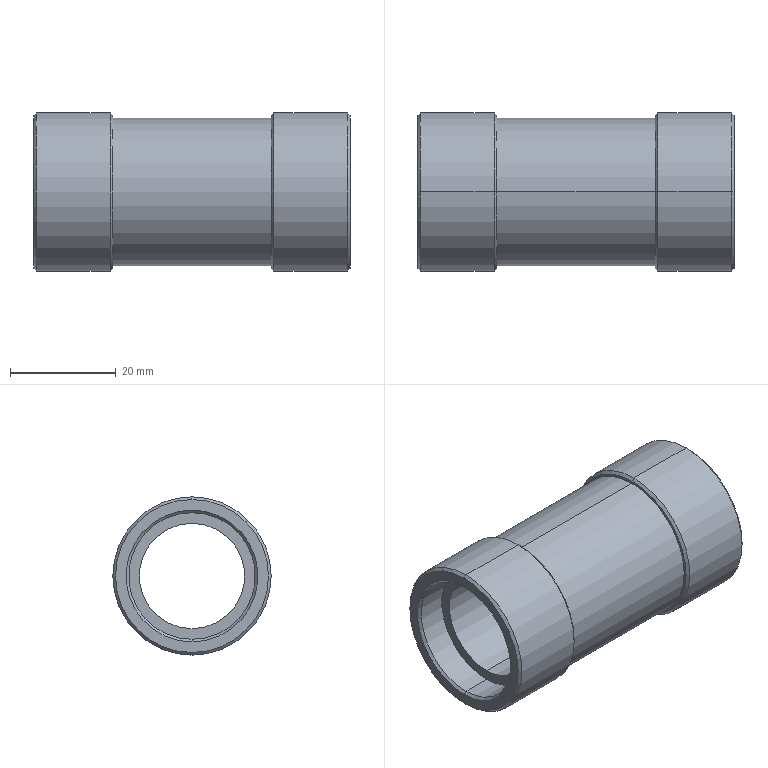Part | SolidWorks | features Chamfer 1, Revolution 1 | 1 solid | 30 faces | box 60 x 30 x 30 mm | volume 19104 mm3 | cone 12 | cylinder 12 | plane 6 | commonest cylinder face diameters 24 x4 30 x4 20 x2 28 x2
STEP:
#1=CARTESIAN_POINT('',(-15.,0.,-14.5));
#2=VERTEX_POINT('',#1);
#3=CARTESIAN_POINT('',(-15.,0.,14.5));
#4=VERTEX_POINT('',#3);
#5=CARTESIAN_POINT('',(-15.,0.,0.));
#6=DIRECTION('',(1.,0.,0.));
#7=DIRECTION('',(0.,0.,1.));
#8=AXIS2_PLACEMENT_3D('',#5,#6,#7);
#9=CIRCLE('',#8,14.5);
#10=EDGE_CURVE('',#2,#4,#9,.T.);
#11=ORIENTED_EDGE('',*,*,#10,.F.);
#12=CARTESIAN_POINT('',(-15.5,0.,-15.));
#13=VERTEX_POINT('',#12);
#14=CARTESIAN_POINT('',(-15.,0.,-14.5));
#15=DIRECTION('',(-0.7071,0.,-0.7071));
#16=VECTOR('',#15,1000.);
#17=LINE('',#14,#16);
#18=EDGE_CURVE('',#2,#13,#17,.T.);
#19=ORIENTED_EDGE('',*,*,#18,.T.);
#20=CARTESIAN_POINT('',(-15.5,0.,15.));
#21=VERTEX_POINT('',#20);
#22=CARTESIAN_POINT('',(-15.5,0.,0.));
#23=DIRECTION('',(-1.,0.,0.));
#24=DIRECTION('',(0.,0.,1.));
#25=AXIS2_PLACEMENT_3D('',#22,#23,#24);
#26=CIRCLE('',#25,15.);
#27=EDGE_CURVE('',#21,#13,#26,.T.);
#28=ORIENTED_EDGE('',*,*,#27,.F.);
#29=CARTESIAN_POINT('',(-15.,0.,14.5));
#30=DIRECTION('',(-0.7071,0.,0.7071));
#31=VECTOR('',#30,1000.);
#32=LINE('',#29,#31);
#33=EDGE_CURVE('',#4,#21,#32,.T.);
#34=ORIENTED_EDGE('',*,*,#33,.F.);
#35=EDGE_LOOP('',(#11,#19,#28,#34));
#36=FACE_OUTER_BOUND('',#35,.T.);
#37=CARTESIAN_POINT('',(-15.,0.,0.));
#38=DIRECTION('',(-1.,0.,0.));
#39=DIRECTION('',(0.,0.,1.));
#40=AXIS2_PLACEMENT_3D('',#37,#38,#39);
#41=CONICAL_SURFACE('',#40,14.5,0.7854);
#42=ADVANCED_FACE('',(#36),#41,.T.);
#43=CARTESIAN_POINT('',(15.,0.,14.5));
#44=VERTEX_POINT('',#43);
#45=CARTESIAN_POINT('',(15.,0.,-14.5));
#46=VERTEX_POINT('',#45);
#47=CARTESIAN_POINT('',(15.,0.,0.));
#48=DIRECTION('',(-1.,0.,0.));
#49=DIRECTION('',(0.,0.,1.));
#50=AXIS2_PLACEMENT_3D('',#47,#48,#49);
#51=CIRCLE('',#50,14.5);
#52=EDGE_CURVE('',#44,#46,#51,.T.);
#53=ORIENTED_EDGE('',*,*,#52,.F.);
#54=CARTESIAN_POINT('',(15.5,0.,15.));
#55=VERTEX_POINT('',#54);
#56=CARTESIAN_POINT('',(15.5,0.,15.));
#57=DIRECTION('',(0.7071,0.,0.7071));
#58=VECTOR('',#57,1000.);
#59=LINE('',#56,#58);
#60=EDGE_CURVE('',#44,#55,#59,.T.);
#61=ORIENTED_EDGE('',*,*,#60,.T.);
#62=CARTESIAN_POINT('',(15.5,0.,-15.));
#63=VERTEX_POINT('',#62);
#64=CARTESIAN_POINT('',(15.5,0.,0.));
#65=DIRECTION('',(1.,0.,0.));
#66=DIRECTION('',(0.,0.,1.));
#67=AXIS2_PLACEMENT_3D('',#64,#65,#66);
#68=CIRCLE('',#67,15.);
#69=EDGE_CURVE('',#63,#55,#68,.T.);
#70=ORIENTED_EDGE('',*,*,#69,.F.);
#71=CARTESIAN_POINT('',(15.5,0.,-15.));
#72=DIRECTION('',(0.7071,0.,-0.7071));
#73=VECTOR('',#72,1000.);
#74=LINE('',#71,#73);
#75=EDGE_CURVE('',#46,#63,#74,.T.);
#76=ORIENTED_EDGE('',*,*,#75,.F.);
#77=EDGE_LOOP('',(#53,#61,#70,#76));
#78=FACE_OUTER_BOUND('',#77,.T.);
#79=CARTESIAN_POINT('',(15.5,0.,0.));
#80=DIRECTION('',(1.,0.,0.));
#81=DIRECTION('',(0.,0.,-1.));
#82=AXIS2_PLACEMENT_3D('',#79,#80,#81);
#83=CONICAL_SURFACE('',#82,15.,0.7854);
#84=ADVANCED_FACE('',(#78),#83,.T.);
#85=CARTESIAN_POINT('',(-30.,0.,14.5));
#86=VERTEX_POINT('',#85);
#87=CARTESIAN_POINT('',(-30.,0.,-14.5));
#88=VERTEX_POINT('',#87);
#89=CARTESIAN_POINT('',(-30.,0.,0.));
#90=DIRECTION('',(-1.,0.,0.));
#91=DIRECTION('',(0.,0.,-1.));
#92=AXIS2_PLACEMENT_3D('',#89,#90,#91);
#93=CIRCLE('',#92,14.5);
#94=EDGE_CURVE('',#86,#88,#93,.T.);
#95=ORIENTED_EDGE('',*,*,#94,.F.);
#96=CARTESIAN_POINT('',(-29.5,0.,15.));
#97=VERTEX_POINT('',#96);
#98=CARTESIAN_POINT('',(-29.5,0.,15.));
#99=DIRECTION('',(0.7071,0.,0.7071));
#100=VECTOR('',#99,1000.);
#101=LINE('',#98,#100);
#102=EDGE_CURVE('',#86,#97,#101,.T.);
#103=ORIENTED_EDGE('',*,*,#102,.T.);
#104=CARTESIAN_POINT('',(-29.5,0.,-15.));
#105=VERTEX_POINT('',#104);
#106=CARTESIAN_POINT('',(-29.5,0.,0.));
#107=DIRECTION('',(1.,0.,0.));
#108=DIRECTION('',(0.,0.,-1.));
#109=AXIS2_PLACEMENT_3D('',#106,#107,#108);
#110=CIRCLE('',#109,15.);
#111=EDGE_CURVE('',#105,#97,#110,.T.);
#112=ORIENTED_EDGE('',*,*,#111,.F.);
#113=CARTESIAN_POINT('',(-29.5,0.,-15.));
#114=DIRECTION('',(0.7071,0.,-0.7071));
#115=VECTOR('',#114,1000.);
#116=LINE('',#113,#115);
#117=EDGE_CURVE('',#88,#105,#116,.T.);
#118=ORIENTED_EDGE('',*,*,#117,.F.);
#119=EDGE_LOOP('',(#95,#103,#112,#118));
#120=FACE_OUTER_BOUND('',#119,.T.);
#121=CARTESIAN_POINT('',(-29.5,0.,0.));
#122=DIRECTION('',(1.,0.,0.));
#123=DIRECTION('',(0.,0.,-1.));
#124=AXIS2_PLACEMENT_3D('',#121,#122,#123);
#125=CONICAL_SURFACE('',#124,15.,0.7854);
#126=ADVANCED_FACE('',(#120),#125,.T.);
#127=CARTESIAN_POINT('',(-29.5,0.,-12.));
#128=VERTEX_POINT('',#127);
#129=CARTESIAN_POINT('',(-29.5,0.,12.));
#130=VERTEX_POINT('',#129);
#131=CARTESIAN_POINT('',(-29.5,0.,0.));
#132=DIRECTION('',(-1.,0.,0.));
#133=DIRECTION('',(0.,0.,-1.));
#134=AXIS2_PLACEMENT_3D('',#131,#132,#133);
#135=CIRCLE('',#134,12.);
#136=EDGE_CURVE('',#128,#130,#135,.T.);
#137=ORIENTED_EDGE('',*,*,#136,.F.);
#138=CARTESIAN_POINT('',(-30.,0.,-12.5));
#139=VERTEX_POINT('',#138);
#140=CARTESIAN_POINT('',(-30.,0.,-12.5));
#141=DIRECTION('',(-0.7071,0.,-0.7071));
#142=VECTOR('',#141,1000.);
#143=LINE('',#140,#142);
#144=EDGE_CURVE('',#128,#139,#143,.T.);
#145=ORIENTED_EDGE('',*,*,#144,.T.);
#146=CARTESIAN_POINT('',(-30.,0.,12.5));
#147=VERTEX_POINT('',#146);
#148=CARTESIAN_POINT('',(-30.,0.,0.));
#149=DIRECTION('',(1.,0.,0.));
#150=DIRECTION('',(0.,0.,-1.));
#151=AXIS2_PLACEMENT_3D('',#148,#149,#150);
#152=CIRCLE('',#151,12.5);
#153=EDGE_CURVE('',#147,#139,#152,.T.);
#154=ORIENTED_EDGE('',*,*,#153,.F.);
#155=CARTESIAN_POINT('',(-30.,0.,12.5));
#156=DIRECTION('',(-0.7071,0.,0.7071));
#157=VECTOR('',#156,1000.);
#158=LINE('',#155,#157);
#159=EDGE_CURVE('',#130,#147,#158,.T.);
#160=ORIENTED_EDGE('',*,*,#159,.F.);
#161=EDGE_LOOP('',(#137,#145,#154,#160));
#162=FACE_OUTER_BOUND('',#161,.T.);
#163=CARTESIAN_POINT('',(-30.,0.,0.));
#164=DIRECTION('',(-1.,0.,0.));
#165=DIRECTION('',(0.,0.,1.));
#166=AXIS2_PLACEMENT_3D('',#163,#164,#165);
#167=CONICAL_SURFACE('',#166,12.5,0.7854);
#168=ADVANCED_FACE('',(#162),#167,.F.);
#169=CARTESIAN_POINT('',(30.,0.,-14.5));
#170=VERTEX_POINT('',#169);
#171=CARTESIAN_POINT('',(30.,0.,14.5));
#172=VERTEX_POINT('',#171);
#173=CARTESIAN_POINT('',(30.,0.,0.));
#174=DIRECTION('',(1.,0.,0.));
#175=DIRECTION('',(0.,0.,-1.));
#176=AXIS2_PLACEMENT_3D('',#173,#174,#175);
#177=CIRCLE('',#176,14.5);
#178=EDGE_CURVE('',#170,#172,#177,.T.);
#179=ORIENTED_EDGE('',*,*,#178,.F.);
#180=CARTESIAN_POINT('',(29.5,0.,-15.));
#181=VERTEX_POINT('',#180);
#182=CARTESIAN_POINT('',(30.,0.,-14.5));
#183=DIRECTION('',(-0.7071,0.,-0.7071));
#184=VECTOR('',#183,1000.);
#185=LINE('',#182,#184);
#186=EDGE_CURVE('',#170,#181,#185,.T.);
#187=ORIENTED_EDGE('',*,*,#186,.T.);
#188=CARTESIAN_POINT('',(29.5,0.,15.));
#189=VERTEX_POINT('',#188);
#190=CARTESIAN_POINT('',(29.5,0.,0.));
#191=DIRECTION('',(-1.,0.,0.));
#192=DIRECTION('',(0.,0.,-1.));
#193=AXIS2_PLACEMENT_3D('',#190,#191,#192);
#194=CIRCLE('',#193,15.);
#195=EDGE_CURVE('',#189,#181,#194,.T.);
#196=ORIENTED_EDGE('',*,*,#195,.F.);
#197=CARTESIAN_POINT('',(30.,0.,14.5));
#198=DIRECTION('',(-0.7071,0.,0.7071));
#199=VECTOR('',#198,1000.);
#200=LINE('',#197,#199);
#201=EDGE_CURVE('',#172,#189,#200,.T.);
#202=ORIENTED_EDGE('',*,*,#201,.F.);
#203=EDGE_LOOP('',(#179,#187,#196,#202));
#204=FACE_OUTER_BOUND('',#203,.T.);
#205=CARTESIAN_POINT('',(30.,0.,0.));
#206=DIRECTION('',(-1.,0.,0.));
#207=DIRECTION('',(0.,0.,1.));
#208=AXIS2_PLACEMENT_3D('',#205,#206,#207);
#209=CONICAL_SURFACE('',#208,14.5,0.7854);
#210=ADVANCED_FACE('',(#204),#209,.T.);
#211=CARTESIAN_POINT('',(29.5,0.,12.));
#212=VERTEX_POINT('',#211);
#213=CARTESIAN_POINT('',(29.5,0.,-12.));
#214=VERTEX_POINT('',#213);
#215=CARTESIAN_POINT('',(29.5,0.,0.));
#216=DIRECTION('',(1.,0.,0.));
#217=DIRECTION('',(0.,0.,-1.));
#218=AXIS2_PLACEMENT_3D('',#215,#216,#217);
#219=CIRCLE('',#218,12.);
#220=EDGE_CURVE('',#212,#214,#219,.T.);
#221=ORIENTED_EDGE('',*,*,#220,.F.);
#222=CARTESIAN_POINT('',(30.,0.,12.5));
#223=VERTEX_POINT('',#222);
#224=CARTESIAN_POINT('',(29.5,0.,12.));
#225=DIRECTION('',(0.7071,0.,0.7071));
#226=VECTOR('',#225,1000.);
#227=LINE('',#224,#226);
#228=EDGE_CURVE('',#212,#223,#227,.T.);
#229=ORIENTED_EDGE('',*,*,#228,.T.);
#230=CARTESIAN_POINT('',(30.,0.,-12.5));
#231=VERTEX_POINT('',#230);
#232=CARTESIAN_POINT('',(30.,0.,0.));
#233=DIRECTION('',(-1.,0.,0.));
#234=DIRECTION('',(0.,0.,-1.));
#235=AXIS2_PLACEMENT_3D('',#232,#233,#234);
#236=CIRCLE('',#235,12.5);
#237=EDGE_CURVE('',#231,#223,#236,.T.);
#238=ORIENTED_EDGE('',*,*,#237,.F.);
#239=CARTESIAN_POINT('',(29.5,0.,-12.));
#240=DIRECTION('',(0.7071,0.,-0.7071));
#241=VECTOR('',#240,1000.);
#242=LINE('',#239,#241);
#243=EDGE_CURVE('',#214,#231,#242,.T.);
#244=ORIENTED_EDGE('',*,*,#243,.F.);
#245=EDGE_LOOP('',(#221,#229,#238,#244));
#246=FACE_OUTER_BOUND('',#245,.T.);
#247=CARTESIAN_POINT('',(29.5,0.,0.));
#248=DIRECTION('',(1.,0.,0.));
#249=DIRECTION('',(0.,0.,-1.));
#250=AXIS2_PLACEMENT_3D('',#247,#248,#249);
#251=CONICAL_SURFACE('',#250,12.,0.7854);
#252=ADVANCED_FACE('',(#246),#251,.F.);
#253=CARTESIAN_POINT('',(24.,0.,12.));
#254=VERTEX_POINT('',#253);
#255=CARTESIAN_POINT('',(24.,0.,-12.));
#256=VERTEX_POINT('',#255);
#257=CARTESIAN_POINT('',(24.,0.,0.));
#258=DIRECTION('',(1.,0.,0.));
#259=DIRECTION('',(0.,0.,-1.));
#260=AXIS2_PLACEMENT_3D('',#257,#258,#259);
#261=CIRCLE('',#260,12.);
#262=EDGE_CURVE('',#254,#256,#261,.T.);
#263=ORIENTED_EDGE('',*,*,#262,.F.);
#264=CARTESIAN_POINT('',(48.534,0.,12.));
#265=DIRECTION('',(1.,0.,0.));
#266=VECTOR('',#265,1000.);
#267=LINE('',#264,#266);
#268=EDGE_CURVE('',#254,#212,#267,.T.);
#269=ORIENTED_EDGE('',*,*,#268,.T.);
#270=ORIENTED_EDGE('',*,*,#220,.T.);
#271=CARTESIAN_POINT('',(48.534,0.,-12.));
#272=DIRECTION('',(1.,0.,0.));
#273=VECTOR('',#272,1000.);
#274=LINE('',#271,#273);
#275=EDGE_CURVE('',#256,#214,#274,.T.);
#276=ORIENTED_EDGE('',*,*,#275,.F.);
#277=EDGE_LOOP('',(#263,#269,#270,#276));
#278=FACE_OUTER_BOUND('',#277,.T.);
#279=CARTESIAN_POINT('',(48.534,0.,0.));
#280=DIRECTION('',(1.,0.,0.));
#281=DIRECTION('',(0.,0.,-1.));
#282=AXIS2_PLACEMENT_3D('',#279,#280,#281);
#283=CYLINDRICAL_SURFACE('',#282,12.);
#284=ADVANCED_FACE('',(#278),#283,.F.);
#285=CARTESIAN_POINT('',(-24.,0.,10.));
#286=VERTEX_POINT('',#285);
#287=CARTESIAN_POINT('',(-24.,0.,-10.));
#288=VERTEX_POINT('',#287);
#289=CARTESIAN_POINT('',(-24.,0.,0.));
#290=DIRECTION('',(1.,0.,0.));
#291=DIRECTION('',(0.,0.,-1.));
#292=AXIS2_PLACEMENT_3D('',#289,#290,#291);
#293=CIRCLE('',#292,10.);
#294=EDGE_CURVE('',#286,#288,#293,.T.);
#295=ORIENTED_EDGE('',*,*,#294,.F.);
#296=CARTESIAN_POINT('',(24.,0.,10.));
#297=VERTEX_POINT('',#296);
#298=CARTESIAN_POINT('',(48.534,0.,10.));
#299=DIRECTION('',(1.,0.,0.));
#300=VECTOR('',#299,1000.);
#301=LINE('',#298,#300);
#302=EDGE_CURVE('',#286,#297,#301,.T.);
#303=ORIENTED_EDGE('',*,*,#302,.T.);
#304=CARTESIAN_POINT('',(24.,0.,-10.));
#305=VERTEX_POINT('',#304);
#306=CARTESIAN_POINT('',(24.,0.,0.));
#307=DIRECTION('',(1.,0.,0.));
#308=DIRECTION('',(0.,0.,-1.));
#309=AXIS2_PLACEMENT_3D('',#306,#307,#308);
#310=CIRCLE('',#309,10.);
#311=EDGE_CURVE('',#297,#305,#310,.T.);
#312=ORIENTED_EDGE('',*,*,#311,.T.);
#313=CARTESIAN_POINT('',(48.534,0.,-10.));
#314=DIRECTION('',(1.,0.,0.));
#315=VECTOR('',#314,1000.);
#316=LINE('',#313,#315);
#317=EDGE_CURVE('',#288,#305,#316,.T.);
#318=ORIENTED_EDGE('',*,*,#317,.F.);
#319=EDGE_LOOP('',(#295,#303,#312,#318));
#320=FACE_OUTER_BOUND('',#319,.T.);
#321=CARTESIAN_POINT('',(48.534,0.,0.));
#322=DIRECTION('',(1.,0.,0.));
#323=DIRECTION('',(0.,0.,-1.));
#324=AXIS2_PLACEMENT_3D('',#321,#322,#323);
#325=CYLINDRICAL_SURFACE('',#324,10.);
#326=ADVANCED_FACE('',(#320),#325,.F.);
#327=ORIENTED_EDGE('',*,*,#136,.T.);
#328=CARTESIAN_POINT('',(-24.,0.,12.));
#329=VERTEX_POINT('',#328);
#330=CARTESIAN_POINT('',(48.534,0.,12.));
#331=DIRECTION('',(1.,0.,0.));
#332=VECTOR('',#331,1000.);
#333=LINE('',#330,#332);
#334=EDGE_CURVE('',#130,#329,#333,.T.);
#335=ORIENTED_EDGE('',*,*,#334,.T.);
#336=CARTESIAN_POINT('',(-24.,0.,-12.));
#337=VERTEX_POINT('',#336);
#338=CARTESIAN_POINT('',(-24.,0.,0.));
#339=DIRECTION('',(1.,0.,0.));
#340=DIRECTION('',(0.,0.,-1.));
#341=AXIS2_PLACEMENT_3D('',#338,#339,#340);
#342=CIRCLE('',#341,12.);
#343=EDGE_CURVE('',#329,#337,#342,.T.);
#344=ORIENTED_EDGE('',*,*,#343,.T.);
#345=CARTESIAN_POINT('',(48.534,0.,-12.));
#346=DIRECTION('',(1.,0.,0.));
#347=VECTOR('',#346,1000.);
#348=LINE('',#345,#347);
#349=EDGE_CURVE('',#128,#337,#348,.T.);
#350=ORIENTED_EDGE('',*,*,#349,.F.);
#351=EDGE_LOOP('',(#327,#335,#344,#350));
#352=FACE_OUTER_BOUND('',#351,.T.);
#353=CARTESIAN_POINT('',(48.534,0.,0.));
#354=DIRECTION('',(1.,0.,0.));
#355=DIRECTION('',(0.,0.,-1.));
#356=AXIS2_PLACEMENT_3D('',#353,#354,#355);
#357=CYLINDRICAL_SURFACE('',#356,12.);
#358=ADVANCED_FACE('',(#352),#357,.F.);
#359=ORIENTED_EDGE('',*,*,#111,.T.);
#360=CARTESIAN_POINT('',(48.534,0.,15.));
#361=DIRECTION('',(1.,0.,0.));
#362=VECTOR('',#361,1000.);
#363=LINE('',#360,#362);
#364=EDGE_CURVE('',#97,#21,#363,.T.);
#365=ORIENTED_EDGE('',*,*,#364,.T.);
#366=ORIENTED_EDGE('',*,*,#27,.T.);
#367=CARTESIAN_POINT('',(48.534,0.,-15.));
#368=DIRECTION('',(1.,0.,0.));
#369=VECTOR('',#368,1000.);
#370=LINE('',#367,#369);
#371=EDGE_CURVE('',#105,#13,#370,.T.);
#372=ORIENTED_EDGE('',*,*,#371,.F.);
#373=EDGE_LOOP('',(#359,#365,#366,#372));
#374=FACE_OUTER_BOUND('',#373,.T.);
#375=CARTESIAN_POINT('',(48.534,0.,0.));
#376=DIRECTION('',(1.,0.,0.));
#377=DIRECTION('',(0.,0.,-1.));
#378=AXIS2_PLACEMENT_3D('',#375,#376,#377);
#379=CYLINDRICAL_SURFACE('',#378,15.);
#380=ADVANCED_FACE('',(#374),#379,.T.);
#381=CARTESIAN_POINT('',(-15.,0.,-14.));
#382=VERTEX_POINT('',#381);
#383=CARTESIAN_POINT('',(-15.,0.,14.));
#384=VERTEX_POINT('',#383);
#385=CARTESIAN_POINT('',(-15.,0.,0.));
#386=DIRECTION('',(1.,0.,0.));
#387=DIRECTION('',(0.,0.,-1.));
#388=AXIS2_PLACEMENT_3D('',#385,#386,#387);
#389=CIRCLE('',#388,14.);
#390=EDGE_CURVE('',#382,#384,#389,.T.);
#391=ORIENTED_EDGE('',*,*,#390,.T.);
#392=CARTESIAN_POINT('',(15.,0.,14.));
#393=VERTEX_POINT('',#392);
#394=CARTESIAN_POINT('',(48.534,0.,14.));
#395=DIRECTION('',(1.,0.,0.));
#396=VECTOR('',#395,1000.);
#397=LINE('',#394,#396);
#398=EDGE_CURVE('',#384,#393,#397,.T.);
#399=ORIENTED_EDGE('',*,*,#398,.T.);
#400=CARTESIAN_POINT('',(15.,0.,-14.));
#401=VERTEX_POINT('',#400);
#402=CARTESIAN_POINT('',(15.,0.,0.));
#403=DIRECTION('',(1.,0.,0.));
#404=DIRECTION('',(0.,0.,-1.));
#405=AXIS2_PLACEMENT_3D('',#402,#403,#404);
#406=CIRCLE('',#405,14.);
#407=EDGE_CURVE('',#401,#393,#406,.T.);
#408=ORIENTED_EDGE('',*,*,#407,.F.);
#409=CARTESIAN_POINT('',(48.534,0.,-14.));
#410=DIRECTION('',(1.,0.,0.));
#411=VECTOR('',#410,1000.);
#412=LINE('',#409,#411);
#413=EDGE_CURVE('',#382,#401,#412,.T.);
#414=ORIENTED_EDGE('',*,*,#413,.F.);
#415=EDGE_LOOP('',(#391,#399,#408,#414));
#416=FACE_OUTER_BOUND('',#415,.T.);
#417=CARTESIAN_POINT('',(48.534,0.,0.));
#418=DIRECTION('',(1.,0.,0.));
#419=DIRECTION('',(0.,0.,-1.));
#420=AXIS2_PLACEMENT_3D('',#417,#418,#419);
#421=CYLINDRICAL_SURFACE('',#420,14.);
#422=ADVANCED_FACE('',(#416),#421,.T.);
#423=ORIENTED_EDGE('',*,*,#69,.T.);
#424=CARTESIAN_POINT('',(48.534,0.,15.));
#425=DIRECTION('',(1.,0.,0.));
#426=VECTOR('',#425,1000.);
#427=LINE('',#424,#426);
#428=EDGE_CURVE('',#55,#189,#427,.T.);
#429=ORIENTED_EDGE('',*,*,#428,.T.);
#430=ORIENTED_EDGE('',*,*,#195,.T.);
#431=CARTESIAN_POINT('',(48.534,0.,-15.));
#432=DIRECTION('',(1.,0.,0.));
#433=VECTOR('',#432,1000.);
#434=LINE('',#431,#433);
#435=EDGE_CURVE('',#63,#181,#434,.T.);
#436=ORIENTED_EDGE('',*,*,#435,.F.);
#437=EDGE_LOOP('',(#423,#429,#430,#436));
#438=FACE_OUTER_BOUND('',#437,.T.);
#439=CARTESIAN_POINT('',(48.534,0.,0.));
#440=DIRECTION('',(1.,0.,0.));
#441=DIRECTION('',(0.,0.,-1.));
#442=AXIS2_PLACEMENT_3D('',#439,#440,#441);
#443=CYLINDRICAL_SURFACE('',#442,15.);
#444=ADVANCED_FACE('',(#438),#443,.T.);
#445=ORIENTED_EDGE('',*,*,#428,.F.);
#446=CARTESIAN_POINT('',(15.5,0.,0.));
#447=DIRECTION('',(1.,0.,0.));
#448=DIRECTION('',(0.,0.,1.));
#449=AXIS2_PLACEMENT_3D('',#446,#447,#448);
#450=CIRCLE('',#449,15.);
#451=EDGE_CURVE('',#55,#63,#450,.T.);
#452=ORIENTED_EDGE('',*,*,#451,.T.);
#453=ORIENTED_EDGE('',*,*,#435,.T.);
#454=CARTESIAN_POINT('',(29.5,0.,0.));
#455=DIRECTION('',(-1.,0.,0.));
#456=DIRECTION('',(0.,0.,-1.));
#457=AXIS2_PLACEMENT_3D('',#454,#455,#456);
#458=CIRCLE('',#457,15.);
#459=EDGE_CURVE('',#181,#189,#458,.T.);
#460=ORIENTED_EDGE('',*,*,#459,.T.);
#461=EDGE_LOOP('',(#445,#452,#453,#460));
#462=FACE_OUTER_BOUND('',#461,.T.);
#463=CARTESIAN_POINT('',(48.534,0.,0.));
#464=DIRECTION('',(1.,0.,0.));
#465=DIRECTION('',(0.,0.,-1.));
#466=AXIS2_PLACEMENT_3D('',#463,#464,#465);
#467=CYLINDRICAL_SURFACE('',#466,15.);
#468=ADVANCED_FACE('',(#462),#467,.T.);
#469=CARTESIAN_POINT('',(15.,0.,0.));
#470=DIRECTION('',(-1.,0.,0.));
#471=DIRECTION('',(0.,0.,1.));
#472=AXIS2_PLACEMENT_3D('',#469,#470,#471);
#473=CIRCLE('',#472,14.5);
#474=EDGE_CURVE('',#46,#44,#473,.T.);
#475=ORIENTED_EDGE('',*,*,#474,.T.);
#476=ORIENTED_EDGE('',*,*,#52,.T.);
#477=EDGE_LOOP('',(#475,#476));
#478=FACE_OUTER_BOUND('',#477,.T.);
#479=ORIENTED_EDGE('',*,*,#407,.T.);
#480=CARTESIAN_POINT('',(15.,0.,0.));
#481=DIRECTION('',(1.,0.,0.));
#482=DIRECTION('',(0.,0.,-1.));
#483=AXIS2_PLACEMENT_3D('',#480,#481,#482);
#484=CIRCLE('',#483,14.);
#485=EDGE_CURVE('',#393,#401,#484,.T.);
#486=ORIENTED_EDGE('',*,*,#485,.T.);
#487=EDGE_LOOP('',(#479,#486));
#488=FACE_BOUND('',#487,.T.);
#489=CARTESIAN_POINT('',(15.,0.,0.));
#490=DIRECTION('',(-1.,0.,0.));
#491=DIRECTION('',(0.,0.,1.));
#492=AXIS2_PLACEMENT_3D('',#489,#490,#491);
#493=PLANE('',#492);
#494=ADVANCED_FACE('',(#478,#488),#493,.T.);
#495=ORIENTED_EDGE('',*,*,#398,.F.);
#496=CARTESIAN_POINT('',(-15.,0.,0.));
#497=DIRECTION('',(1.,0.,0.));
#498=DIRECTION('',(0.,0.,-1.));
#499=AXIS2_PLACEMENT_3D('',#496,#497,#498);
#500=CIRCLE('',#499,14.);
#501=EDGE_CURVE('',#384,#382,#500,.T.);
#502=ORIENTED_EDGE('',*,*,#501,.T.);
#503=ORIENTED_EDGE('',*,*,#413,.T.);
#504=ORIENTED_EDGE('',*,*,#485,.F.);
#505=EDGE_LOOP('',(#495,#502,#503,#504));
#506=FACE_OUTER_BOUND('',#505,.T.);
#507=CARTESIAN_POINT('',(48.534,0.,0.));
#508=DIRECTION('',(1.,0.,0.));
#509=DIRECTION('',(0.,0.,-1.));
#510=AXIS2_PLACEMENT_3D('',#507,#508,#509);
#511=CYLINDRICAL_SURFACE('',#510,14.);
#512=ADVANCED_FACE('',(#506),#511,.T.);
#513=CARTESIAN_POINT('',(-15.,0.,0.));
#514=DIRECTION('',(1.,0.,0.));
#515=DIRECTION('',(0.,0.,1.));
#516=AXIS2_PLACEMENT_3D('',#513,#514,#515);
#517=CIRCLE('',#516,14.5);
#518=EDGE_CURVE('',#4,#2,#517,.T.);
#519=ORIENTED_EDGE('',*,*,#518,.T.);
#520=ORIENTED_EDGE('',*,*,#10,.T.);
#521=EDGE_LOOP('',(#519,#520));
#522=FACE_OUTER_BOUND('',#521,.T.);
#523=ORIENTED_EDGE('',*,*,#390,.F.);
#524=ORIENTED_EDGE('',*,*,#501,.F.);
#525=EDGE_LOOP('',(#523,#524));
#526=FACE_BOUND('',#525,.T.);
#527=CARTESIAN_POINT('',(-15.,0.,0.));
#528=DIRECTION('',(-1.,0.,0.));
#529=DIRECTION('',(0.,0.,1.));
#530=AXIS2_PLACEMENT_3D('',#527,#528,#529);
#531=PLANE('',#530);
#532=ADVANCED_FACE('',(#522,#526),#531,.F.);
#533=ORIENTED_EDGE('',*,*,#364,.F.);
#534=CARTESIAN_POINT('',(-29.5,0.,0.));
#535=DIRECTION('',(1.,0.,0.));
#536=DIRECTION('',(0.,0.,-1.));
#537=AXIS2_PLACEMENT_3D('',#534,#535,#536);
#538=CIRCLE('',#537,15.);
#539=EDGE_CURVE('',#97,#105,#538,.T.);
#540=ORIENTED_EDGE('',*,*,#539,.T.);
#541=ORIENTED_EDGE('',*,*,#371,.T.);
#542=CARTESIAN_POINT('',(-15.5,0.,0.));
#543=DIRECTION('',(-1.,0.,0.));
#544=DIRECTION('',(0.,0.,1.));
#545=AXIS2_PLACEMENT_3D('',#542,#543,#544);
#546=CIRCLE('',#545,15.);
#547=EDGE_CURVE('',#13,#21,#546,.T.);
#548=ORIENTED_EDGE('',*,*,#547,.T.);
#549=EDGE_LOOP('',(#533,#540,#541,#548));
#550=FACE_OUTER_BOUND('',#549,.T.);
#551=CARTESIAN_POINT('',(48.534,0.,0.));
#552=DIRECTION('',(1.,0.,0.));
#553=DIRECTION('',(0.,0.,-1.));
#554=AXIS2_PLACEMENT_3D('',#551,#552,#553);
#555=CYLINDRICAL_SURFACE('',#554,15.);
#556=ADVANCED_FACE('',(#550),#555,.T.);
#557=ORIENTED_EDGE('',*,*,#153,.T.);
#558=CARTESIAN_POINT('',(-30.,0.,0.));
#559=DIRECTION('',(1.,0.,0.));
#560=DIRECTION('',(0.,0.,-1.));
#561=AXIS2_PLACEMENT_3D('',#558,#559,#560);
#562=CIRCLE('',#561,12.5);
#563=EDGE_CURVE('',#139,#147,#562,.T.);
#564=ORIENTED_EDGE('',*,*,#563,.T.);
#565=EDGE_LOOP('',(#557,#564));
#566=FACE_BOUND('',#565,.T.);
#567=CARTESIAN_POINT('',(-30.,0.,0.));
#568=DIRECTION('',(-1.,0.,0.));
#569=DIRECTION('',(0.,0.,-1.));
#570=AXIS2_PLACEMENT_3D('',#567,#568,#569);
#571=CIRCLE('',#570,14.5);
#572=EDGE_CURVE('',#88,#86,#571,.T.);
#573=ORIENTED_EDGE('',*,*,#572,.T.);
#574=ORIENTED_EDGE('',*,*,#94,.T.);
#575=EDGE_LOOP('',(#573,#574));
#576=FACE_OUTER_BOUND('',#575,.T.);
#577=CARTESIAN_POINT('',(-30.,0.,0.));
#578=DIRECTION('',(1.,0.,0.));
#579=DIRECTION('',(0.,0.,-1.));
#580=AXIS2_PLACEMENT_3D('',#577,#578,#579);
#581=PLANE('',#580);
#582=ADVANCED_FACE('',(#566,#576),#581,.F.);
#583=ORIENTED_EDGE('',*,*,#334,.F.);
#584=CARTESIAN_POINT('',(-29.5,0.,0.));
#585=DIRECTION('',(-1.,0.,0.));
#586=DIRECTION('',(0.,0.,-1.));
#587=AXIS2_PLACEMENT_3D('',#584,#585,#586);
#588=CIRCLE('',#587,12.);
#589=EDGE_CURVE('',#130,#128,#588,.T.);
#590=ORIENTED_EDGE('',*,*,#589,.T.);
#591=ORIENTED_EDGE('',*,*,#349,.T.);
#592=CARTESIAN_POINT('',(-24.,0.,0.));
#593=DIRECTION('',(1.,0.,0.));
#594=DIRECTION('',(0.,0.,-1.));
#595=AXIS2_PLACEMENT_3D('',#592,#593,#594);
#596=CIRCLE('',#595,12.);
#597=EDGE_CURVE('',#337,#329,#596,.T.);
#598=ORIENTED_EDGE('',*,*,#597,.T.);
#599=EDGE_LOOP('',(#583,#590,#591,#598));
#600=FACE_OUTER_BOUND('',#599,.T.);
#601=CARTESIAN_POINT('',(48.534,0.,0.));
#602=DIRECTION('',(1.,0.,0.));
#603=DIRECTION('',(0.,0.,-1.));
#604=AXIS2_PLACEMENT_3D('',#601,#602,#603);
#605=CYLINDRICAL_SURFACE('',#604,12.);
#606=ADVANCED_FACE('',(#600),#605,.F.);
#607=ORIENTED_EDGE('',*,*,#597,.F.);
#608=ORIENTED_EDGE('',*,*,#343,.F.);
#609=EDGE_LOOP('',(#607,#608));
#610=FACE_OUTER_BOUND('',#609,.T.);
#611=CARTESIAN_POINT('',(-24.,0.,0.));
#612=DIRECTION('',(1.,0.,0.));
#613=DIRECTION('',(0.,0.,-1.));
#614=AXIS2_PLACEMENT_3D('',#611,#612,#613);
#615=CIRCLE('',#614,10.);
#616=EDGE_CURVE('',#288,#286,#615,.T.);
#617=ORIENTED_EDGE('',*,*,#616,.T.);
#618=ORIENTED_EDGE('',*,*,#294,.T.);
#619=EDGE_LOOP('',(#617,#618));
#620=FACE_BOUND('',#619,.T.);
#621=CARTESIAN_POINT('',(-24.,0.,0.));
#622=DIRECTION('',(1.,0.,0.));
#623=DIRECTION('',(0.,0.,-1.));
#624=AXIS2_PLACEMENT_3D('',#621,#622,#623);
#625=PLANE('',#624);
#626=ADVANCED_FACE('',(#610,#620),#625,.F.);
#627=ORIENTED_EDGE('',*,*,#302,.F.);
#628=ORIENTED_EDGE('',*,*,#616,.F.);
#629=ORIENTED_EDGE('',*,*,#317,.T.);
#630=CARTESIAN_POINT('',(24.,0.,0.));
#631=DIRECTION('',(1.,0.,0.));
#632=DIRECTION('',(0.,0.,-1.));
#633=AXIS2_PLACEMENT_3D('',#630,#631,#632);
#634=CIRCLE('',#633,10.);
#635=EDGE_CURVE('',#305,#297,#634,.T.);
#636=ORIENTED_EDGE('',*,*,#635,.T.);
#637=EDGE_LOOP('',(#627,#628,#629,#636));
#638=FACE_OUTER_BOUND('',#637,.T.);
#639=CARTESIAN_POINT('',(48.534,0.,0.));
#640=DIRECTION('',(1.,0.,0.));
#641=DIRECTION('',(0.,0.,-1.));
#642=AXIS2_PLACEMENT_3D('',#639,#640,#641);
#643=CYLINDRICAL_SURFACE('',#642,10.);
#644=ADVANCED_FACE('',(#638),#643,.F.);
#645=CARTESIAN_POINT('',(24.,0.,0.));
#646=DIRECTION('',(1.,0.,0.));
#647=DIRECTION('',(0.,0.,-1.));
#648=AXIS2_PLACEMENT_3D('',#645,#646,#647);
#649=CIRCLE('',#648,12.);
#650=EDGE_CURVE('',#256,#254,#649,.T.);
#651=ORIENTED_EDGE('',*,*,#650,.T.);
#652=ORIENTED_EDGE('',*,*,#262,.T.);
#653=EDGE_LOOP('',(#651,#652));
#654=FACE_OUTER_BOUND('',#653,.T.);
#655=ORIENTED_EDGE('',*,*,#635,.F.);
#656=ORIENTED_EDGE('',*,*,#311,.F.);
#657=EDGE_LOOP('',(#655,#656));
#658=FACE_BOUND('',#657,.T.);
#659=CARTESIAN_POINT('',(24.,0.,0.));
#660=DIRECTION('',(1.,0.,0.));
#661=DIRECTION('',(0.,0.,-1.));
#662=AXIS2_PLACEMENT_3D('',#659,#660,#661);
#663=PLANE('',#662);
#664=ADVANCED_FACE('',(#654,#658),#663,.T.);
#665=ORIENTED_EDGE('',*,*,#268,.F.);
#666=ORIENTED_EDGE('',*,*,#650,.F.);
#667=ORIENTED_EDGE('',*,*,#275,.T.);
#668=CARTESIAN_POINT('',(29.5,0.,0.));
#669=DIRECTION('',(1.,0.,0.));
#670=DIRECTION('',(0.,0.,-1.));
#671=AXIS2_PLACEMENT_3D('',#668,#669,#670);
#672=CIRCLE('',#671,12.);
#673=EDGE_CURVE('',#214,#212,#672,.T.);
#674=ORIENTED_EDGE('',*,*,#673,.T.);
#675=EDGE_LOOP('',(#665,#666,#667,#674));
#676=FACE_OUTER_BOUND('',#675,.T.);
#677=CARTESIAN_POINT('',(48.534,0.,0.));
#678=DIRECTION('',(1.,0.,0.));
#679=DIRECTION('',(0.,0.,-1.));
#680=AXIS2_PLACEMENT_3D('',#677,#678,#679);
#681=CYLINDRICAL_SURFACE('',#680,12.);
#682=ADVANCED_FACE('',(#676),#681,.F.);
#683=ORIENTED_EDGE('',*,*,#237,.T.);
#684=CARTESIAN_POINT('',(30.,0.,0.));
#685=DIRECTION('',(-1.,0.,0.));
#686=DIRECTION('',(0.,0.,-1.));
#687=AXIS2_PLACEMENT_3D('',#684,#685,#686);
#688=CIRCLE('',#687,12.5);
#689=EDGE_CURVE('',#223,#231,#688,.T.);
#690=ORIENTED_EDGE('',*,*,#689,.T.);
#691=EDGE_LOOP('',(#683,#690));
#692=FACE_BOUND('',#691,.T.);
#693=CARTESIAN_POINT('',(30.,0.,0.));
#694=DIRECTION('',(1.,0.,0.));
#695=DIRECTION('',(0.,0.,-1.));
#696=AXIS2_PLACEMENT_3D('',#693,#694,#695);
#697=CIRCLE('',#696,14.5);
#698=EDGE_CURVE('',#172,#170,#697,.T.);
#699=ORIENTED_EDGE('',*,*,#698,.T.);
#700=ORIENTED_EDGE('',*,*,#178,.T.);
#701=EDGE_LOOP('',(#699,#700));
#702=FACE_OUTER_BOUND('',#701,.T.);
#703=CARTESIAN_POINT('',(30.,0.,0.));
#704=DIRECTION('',(1.,0.,0.));
#705=DIRECTION('',(0.,0.,-1.));
#706=AXIS2_PLACEMENT_3D('',#703,#704,#705);
#707=PLANE('',#706);
#708=ADVANCED_FACE('',(#692,#702),#707,.T.);
#709=ORIENTED_EDGE('',*,*,#228,.F.);
#710=ORIENTED_EDGE('',*,*,#673,.F.);
#711=ORIENTED_EDGE('',*,*,#243,.T.);
#712=ORIENTED_EDGE('',*,*,#689,.F.);
#713=EDGE_LOOP('',(#709,#710,#711,#712));
#714=FACE_OUTER_BOUND('',#713,.T.);
#715=CARTESIAN_POINT('',(29.5,0.,0.));
#716=DIRECTION('',(1.,0.,0.));
#717=DIRECTION('',(0.,0.,-1.));
#718=AXIS2_PLACEMENT_3D('',#715,#716,#717);
#719=CONICAL_SURFACE('',#718,12.,0.7854);
#720=ADVANCED_FACE('',(#714),#719,.F.);
#721=ORIENTED_EDGE('',*,*,#186,.F.);
#722=ORIENTED_EDGE('',*,*,#698,.F.);
#723=ORIENTED_EDGE('',*,*,#201,.T.);
#724=ORIENTED_EDGE('',*,*,#459,.F.);
#725=EDGE_LOOP('',(#721,#722,#723,#724));
#726=FACE_OUTER_BOUND('',#725,.T.);
#727=CARTESIAN_POINT('',(30.,0.,0.));
#728=DIRECTION('',(-1.,0.,0.));
#729=DIRECTION('',(0.,0.,1.));
#730=AXIS2_PLACEMENT_3D('',#727,#728,#729);
#731=CONICAL_SURFACE('',#730,14.5,0.7854);
#732=ADVANCED_FACE('',(#726),#731,.T.);
#733=ORIENTED_EDGE('',*,*,#144,.F.);
#734=ORIENTED_EDGE('',*,*,#589,.F.);
#735=ORIENTED_EDGE('',*,*,#159,.T.);
#736=ORIENTED_EDGE('',*,*,#563,.F.);
#737=EDGE_LOOP('',(#733,#734,#735,#736));
#738=FACE_OUTER_BOUND('',#737,.T.);
#739=CARTESIAN_POINT('',(-30.,0.,0.));
#740=DIRECTION('',(-1.,0.,0.));
#741=DIRECTION('',(0.,0.,1.));
#742=AXIS2_PLACEMENT_3D('',#739,#740,#741);
#743=CONICAL_SURFACE('',#742,12.5,0.7854);
#744=ADVANCED_FACE('',(#738),#743,.F.);
#745=ORIENTED_EDGE('',*,*,#102,.F.);
#746=ORIENTED_EDGE('',*,*,#572,.F.);
#747=ORIENTED_EDGE('',*,*,#117,.T.);
#748=ORIENTED_EDGE('',*,*,#539,.F.);
#749=EDGE_LOOP('',(#745,#746,#747,#748));
#750=FACE_OUTER_BOUND('',#749,.T.);
#751=CARTESIAN_POINT('',(-29.5,0.,0.));
#752=DIRECTION('',(1.,0.,0.));
#753=DIRECTION('',(0.,0.,-1.));
#754=AXIS2_PLACEMENT_3D('',#751,#752,#753);
#755=CONICAL_SURFACE('',#754,15.,0.7854);
#756=ADVANCED_FACE('',(#750),#755,.T.);
#757=ORIENTED_EDGE('',*,*,#60,.F.);
#758=ORIENTED_EDGE('',*,*,#474,.F.);
#759=ORIENTED_EDGE('',*,*,#75,.T.);
#760=ORIENTED_EDGE('',*,*,#451,.F.);
#761=EDGE_LOOP('',(#757,#758,#759,#760));
#762=FACE_OUTER_BOUND('',#761,.T.);
#763=CARTESIAN_POINT('',(15.5,0.,0.));
#764=DIRECTION('',(1.,0.,0.));
#765=DIRECTION('',(0.,0.,-1.));
#766=AXIS2_PLACEMENT_3D('',#763,#764,#765);
#767=CONICAL_SURFACE('',#766,15.,0.7854);
#768=ADVANCED_FACE('',(#762),#767,.T.);
#769=ORIENTED_EDGE('',*,*,#18,.F.);
#770=ORIENTED_EDGE('',*,*,#518,.F.);
#771=ORIENTED_EDGE('',*,*,#33,.T.);
#772=ORIENTED_EDGE('',*,*,#547,.F.);
#773=EDGE_LOOP('',(#769,#770,#771,#772));
#774=FACE_OUTER_BOUND('',#773,.T.);
#775=CARTESIAN_POINT('',(-15.,0.,0.));
#776=DIRECTION('',(-1.,0.,0.));
#777=DIRECTION('',(0.,0.,1.));
#778=AXIS2_PLACEMENT_3D('',#775,#776,#777);
#779=CONICAL_SURFACE('',#778,14.5,0.7854);
#780=ADVANCED_FACE('',(#774),#779,.T.);
#781=CLOSED_SHELL('',(#42,#84,#126,#168,#210,#252,#284,#326,#358,#380,#422,#444,#468,#494,#512,#532,#556,#582,#606,#626,#644,#664,#682,#708,#720,#732,#744,#756,#768,#780));
#782=MANIFOLD_SOLID_BREP('',#781);
#783=CARTESIAN_POINT('',(0.,0.,0.));
#784=DIRECTION('',(0.,0.,1.));
#785=DIRECTION('',(1.,0.,0.));
#786=AXIS2_PLACEMENT_3D('',#783,#784,#785);
#787=(LENGTH_UNIT()NAMED_UNIT(*)SI_UNIT(.MILLI.,.METRE.));
#788=UNCERTAINTY_MEASURE_WITH_UNIT(LENGTH_MEASURE(0.00001),#787,'','');
#789=(NAMED_UNIT(*)PLANE_ANGLE_UNIT()SI_UNIT($,.RADIAN.));
#790=(NAMED_UNIT(*)SI_UNIT($,.STERADIAN.)SOLID_ANGLE_UNIT());
#791=(GEOMETRIC_REPRESENTATION_CONTEXT(3)GLOBAL_UNCERTAINTY_ASSIGNED_CONTEXT((#788))GLOBAL_UNIT_ASSIGNED_CONTEXT((#787,#789,#790))REPRESENTATION_CONTEXT('',''));
#792=ADVANCED_BREP_SHAPE_REPRESENTATION('',(#782,#786),#791);